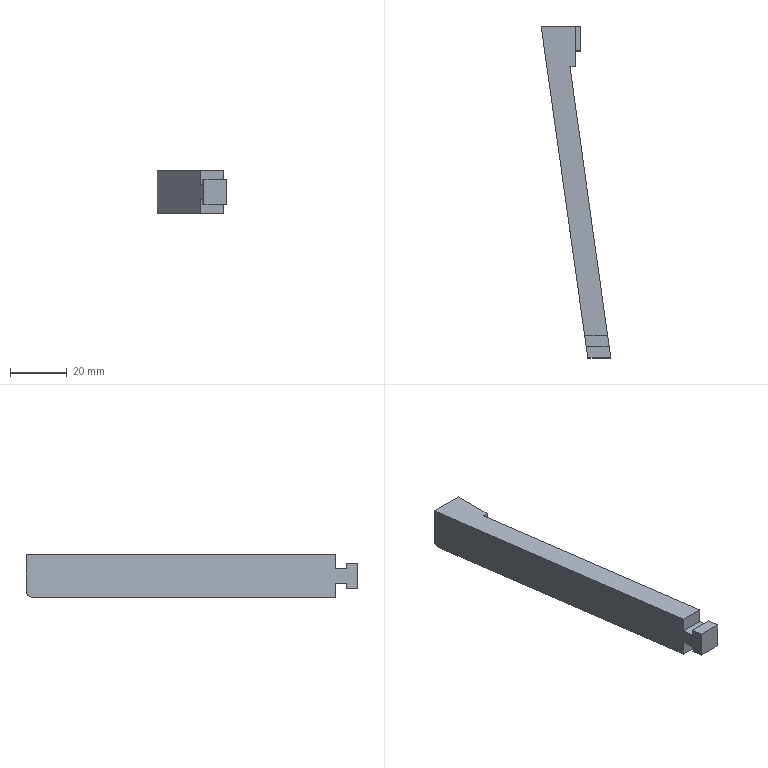Part | STEP file | 1 solid | 27 faces | box 24.479 x 116.693 x 15 mm | volume 14289 mm3 | plane 23 | cylinder 4 | commonest cylinder face diameters 1.005 x2 2.01 x1 4.02 x1